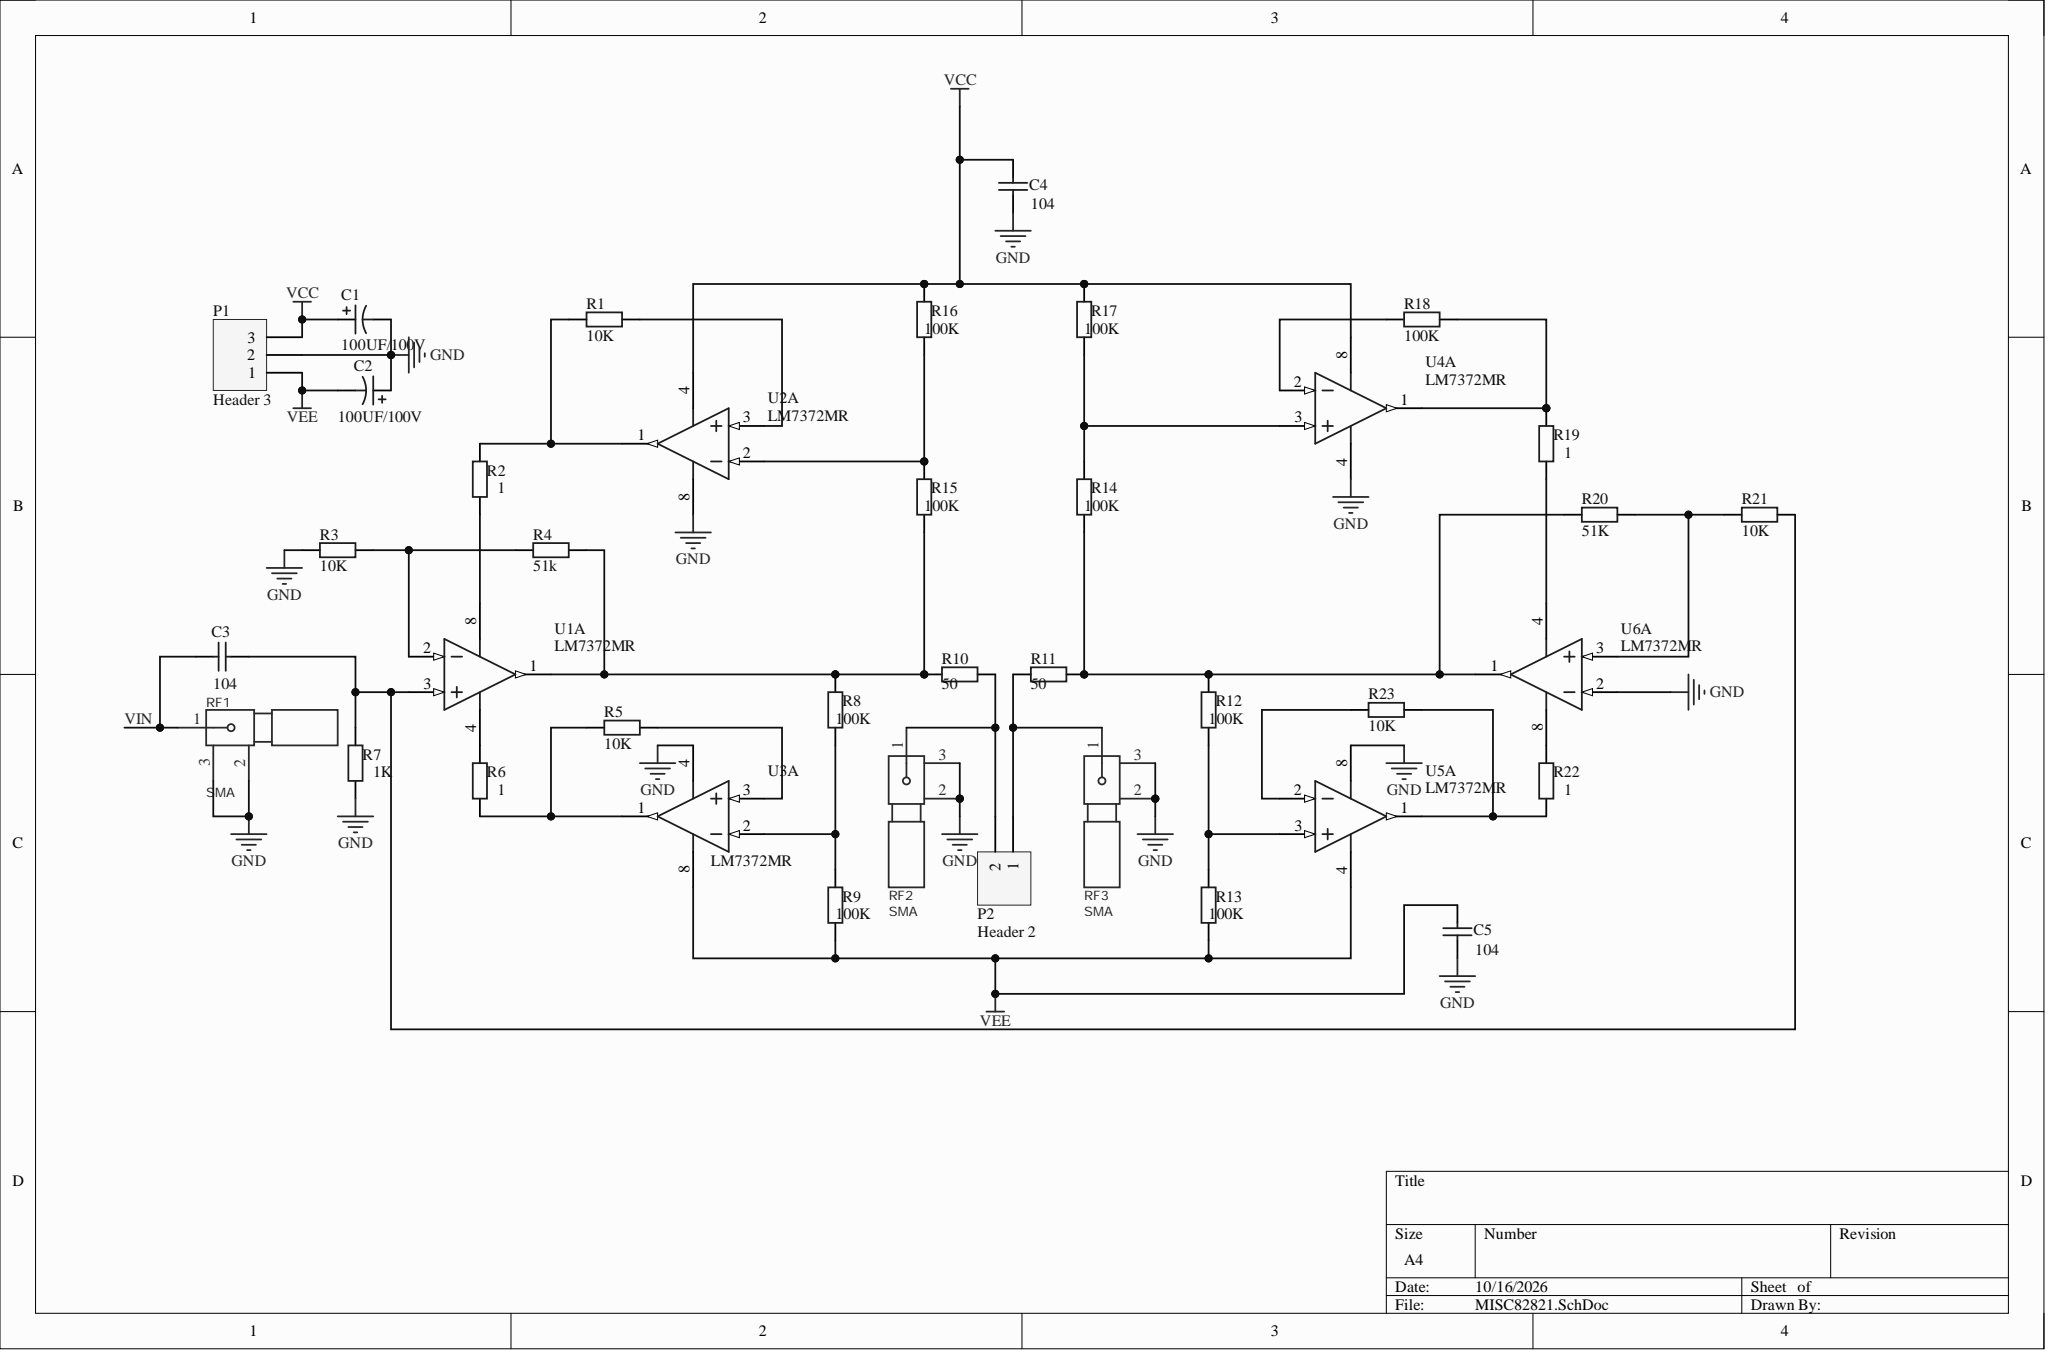Circuit board | Altium Designer | 39 parts | 27 nets
Bill of materials:
Comment,Description,Designator,Footprint,LibRef,Quantity
"100UF/100V","Polarized Capacitor (Surface Mount)","C1, C2","C0805","Cap Pol3","2"
"104","Capacitor (Semiconductor SIM Model)","C3, C4, C5","C1206","Cap Semi","3"
"Header 3","Header, 3-Pin","P1","HDR1X3","Header 3","1"
"Header 2","Header, 2-Pin","P2","HDR1X2","Header 2","1"
"10K","Resistor","R1, R3, R5, R21, R23","AXIAL-0.4","Res2","5"
"1","Resistor","R2, R6, R19, R22","AXIAL-0.4","Res2","4"
"51k","Resistor","R4, R20","AXIAL-0.4","Res2","2"
"1K","Resistor","R7","AXIAL-0.4","Res2","1"
"100K","Resistor","R8, R9, R12, R13, R14, R15, R16, R17, R18","AXIAL-0.4","Res2","9"
"50","Resistor","R10, R11","AXIAL-0.4","Res2","2"
"SMA","Antenna, TI antenna","RF1, RF2, RF3","SMA-SMD_HJ-SMA313","SMB","3"
"LM7372MR","High Speed, High Output Current, Dual Operational Amplifier, 9-pin PSOP","U1, U2, U3, U4, U5, U6","MRA08B_N","LM7372MR","6"
Netlist (Protel format):
[
C1
C0805
100UF/100V



]
[
C2
C0805
100UF/100V



]
[
C3
C1206
104



]
[
C4
C1206
104



]
[
C5
C1206
104



]
[
P1
HDR1X3
Header 3



]
[
P2
HDR1X2
Header 2



]
[
R1
AXIAL-0.4
10K



]
[
R2
AXIAL-0.4
1



]
[
R3
AXIAL-0.4
10K



]
[
R4
AXIAL-0.4
51k



]
[
R5
AXIAL-0.4
10K



]
[
R6
AXIAL-0.4
1



]
[
R7
AXIAL-0.4
1K



]
[
R8
AXIAL-0.4
100K



]
[
R9
AXIAL-0.4
100K



]
[
R10
AXIAL-0.4
50



]
[
R11
AXIAL-0.4
50



]
[
R12
AXIAL-0.4
100K



]
[
R13
AXIAL-0.4
100K



]
[
R14
AXIAL-0.4
100K



]
[
R15
AXIAL-0.4
100K



]
[
R16
AXIAL-0.4
100K



]
[
R17
AXIAL-0.4
100K



]
[
R18
AXIAL-0.4
100K



]
[
R19
AXIAL-0.4
1



]
[
R20
AXIAL-0.4
51K



]
[
R21
AXIAL-0.4
10K



]
[
R22
AXIAL-0.4
1



]
[
R23
AXIAL-0.4
10K



]
[
RF1
SMA-SMD_HJ-SMA313
SMA



]
[
RF2
SMA-SMD_HJ-SMA313
SMA



]
[
RF3
SMA-SMD_HJ-SMA313
SMA



]
[
U1
MRA08B_N
LM7372MR



]
[
U2
MRA08B_N
LM7372MR



]
[
U3
MRA08B_N
LM7372MR



]
[
U4
MRA08B_N
LM7372MR



]
[
U5
MRA08B_N
LM7372MR



]
[
U6
MRA08B_N
LM7372MR



]
(
VIN
C3-2
RF1-1
)
(
VEE
C2-2
C5-2
P1-1
R9-1
R13-1
U3-8
U5-4
)
(
VCC
C1-1
C4-2
P1-3
R16-2
R17-2
U2-4
U4-8
)
(
NetR23_1
R23-1
U5-2
)
(
NetR22_2
R22-2
U6-8
)
(
NetR22_1
R22-1
R23-2
U5-1
)
(
NetR20_2
R20-2
R21-1
U6-3
)
(
NetR19_1
R19-1
U6-4
)
(
NetR18_2
R18-2
R19-2
U4-1
)
(
NetR18_1
R18-1
U4-2
)
(
NetR15_2
R15-2
R16-1
U2-2
)
(
NetR14_2
R14-2
R17-1
U4-3
)
(
NetR12_1
R12-1
R13-2
U5-3
)
(
NetR11_1
R11-1
R12-2
R14-1
R20-1
U6-1
)
(
NetR8_1
R8-1
R9-2
U3-2
)
(
NetR6_2
R6-2
U1-4
)
(
NetR5_2
R5-2
U3-3
)
(
NetR5_1
R5-1
R6-1
U3-1
)
(
NetR4_2
R4-2
R8-2
R10-2
R15-1
U1-1
)
(
NetR3_2
R3-2
R4-1
U1-2
)
(
NetR2_1
R2-1
U1-8
)
(
NetR1_2
R1-2
U2-3
)
(
NetR1_1
R1-1
R2-2
U2-1
)
(
NetP2_2
P2-2
R10-1
RF2-1
)
(
NetP2_1
P2-1
R11-2
RF3-1
)
(
NetC3_1
C3-1
R7-2
R21-2
U1-3
)
(
GND
C1-2
C2-1
C4-1
C5-1
P1-2
R3-1
R7-1
RF1-2
RF1-3
RF2-2
RF2-3
RF3-2
RF3-3
U2-8
U3-4
U4-4
U5-8
U6-2
)